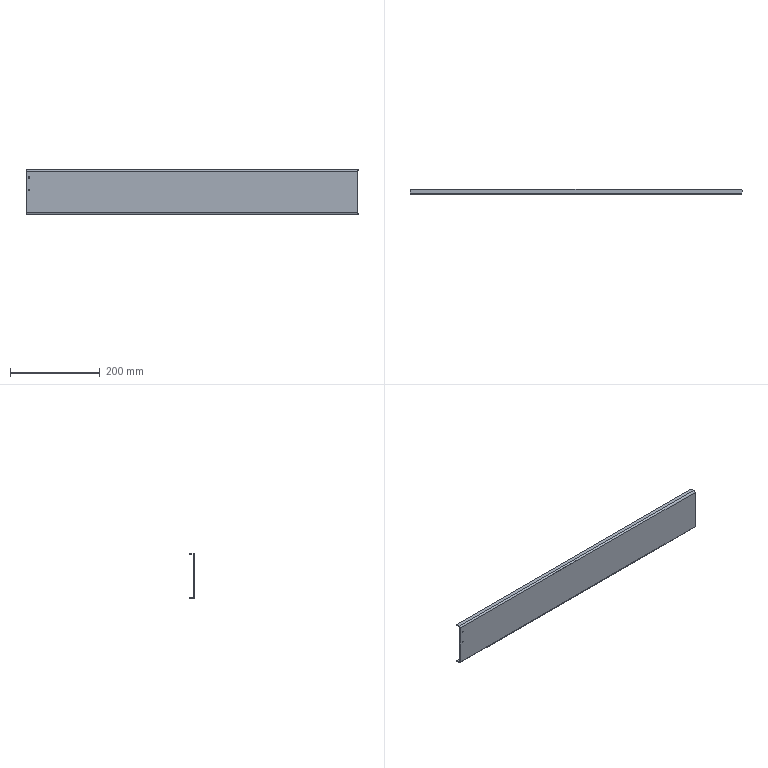Part | SolidWorks | features HoleWzd 2, EdgeFlange 1, Fillet 1, FlatPattern 1, SMBaseFlange 1, SheetMetal 1 | 1 solid | 40 faces | box 740 x 12 x 100 mm | volume 174224 mm3 | cylinder 22 | plane 18 | commonest cylinder face diameters 4.5 x10 3.3 x4 4 x4 3 x2 7 x2
STEP:
#1=CARTESIAN_POINT('',(-363.,-2.,3.35));
#2=VERTEX_POINT('',#1);
#3=CARTESIAN_POINT('',(-363.,-2.,6.65));
#4=VERTEX_POINT('',#3);
#5=CARTESIAN_POINT('',(-363.,-2.,5.));
#6=DIRECTION('',(0.,1.,0.));
#7=DIRECTION('',(0.,0.,1.));
#8=AXIS2_PLACEMENT_3D('',#5,#6,#7);
#9=CIRCLE('',#8,1.65);
#10=EDGE_CURVE('',#2,#4,#9,.T.);
#11=ORIENTED_EDGE('',*,*,#10,.F.);
#12=CARTESIAN_POINT('',(-363.,0.,3.35));
#13=VERTEX_POINT('',#12);
#14=CARTESIAN_POINT('',(-363.,0.,3.35));
#15=DIRECTION('',(0.,1.,0.));
#16=VECTOR('',#15,1000.);
#17=LINE('',#14,#16);
#18=EDGE_CURVE('',#2,#13,#17,.T.);
#19=ORIENTED_EDGE('',*,*,#18,.T.);
#20=CARTESIAN_POINT('',(-363.,0.,6.65));
#21=VERTEX_POINT('',#20);
#22=CARTESIAN_POINT('',(-363.,0.,5.));
#23=DIRECTION('',(0.,1.,0.));
#24=DIRECTION('',(0.,0.,1.));
#25=AXIS2_PLACEMENT_3D('',#22,#23,#24);
#26=CIRCLE('',#25,1.65);
#27=EDGE_CURVE('',#13,#21,#26,.T.);
#28=ORIENTED_EDGE('',*,*,#27,.T.);
#29=CARTESIAN_POINT('',(-363.,0.,6.65));
#30=DIRECTION('',(0.,1.,0.));
#31=VECTOR('',#30,1000.);
#32=LINE('',#29,#31);
#33=EDGE_CURVE('',#4,#21,#32,.T.);
#34=ORIENTED_EDGE('',*,*,#33,.F.);
#35=EDGE_LOOP('',(#11,#19,#28,#34));
#36=FACE_OUTER_BOUND('',#35,.T.);
#37=CARTESIAN_POINT('',(-363.,0.,5.));
#38=DIRECTION('',(0.,1.,0.));
#39=DIRECTION('',(0.,0.,1.));
#40=AXIS2_PLACEMENT_3D('',#37,#38,#39);
#41=CYLINDRICAL_SURFACE('',#40,1.65);
#42=ADVANCED_FACE('',(#36),#41,.F.);
#43=CARTESIAN_POINT('',(-363.,-2.,30.35));
#44=VERTEX_POINT('',#43);
#45=CARTESIAN_POINT('',(-363.,-2.,33.65));
#46=VERTEX_POINT('',#45);
#47=CARTESIAN_POINT('',(-363.,-2.,32.));
#48=DIRECTION('',(0.,1.,0.));
#49=DIRECTION('',(0.,0.,1.));
#50=AXIS2_PLACEMENT_3D('',#47,#48,#49);
#51=CIRCLE('',#50,1.65);
#52=EDGE_CURVE('',#44,#46,#51,.T.);
#53=ORIENTED_EDGE('',*,*,#52,.F.);
#54=CARTESIAN_POINT('',(-363.,0.,30.35));
#55=VERTEX_POINT('',#54);
#56=CARTESIAN_POINT('',(-363.,0.,30.35));
#57=DIRECTION('',(0.,1.,0.));
#58=VECTOR('',#57,1000.);
#59=LINE('',#56,#58);
#60=EDGE_CURVE('',#44,#55,#59,.T.);
#61=ORIENTED_EDGE('',*,*,#60,.T.);
#62=CARTESIAN_POINT('',(-363.,0.,33.65));
#63=VERTEX_POINT('',#62);
#64=CARTESIAN_POINT('',(-363.,0.,32.));
#65=DIRECTION('',(0.,1.,0.));
#66=DIRECTION('',(0.,0.,1.));
#67=AXIS2_PLACEMENT_3D('',#64,#65,#66);
#68=CIRCLE('',#67,1.65);
#69=EDGE_CURVE('',#55,#63,#68,.T.);
#70=ORIENTED_EDGE('',*,*,#69,.T.);
#71=CARTESIAN_POINT('',(-363.,0.,33.65));
#72=DIRECTION('',(0.,1.,0.));
#73=VECTOR('',#72,1000.);
#74=LINE('',#71,#73);
#75=EDGE_CURVE('',#46,#63,#74,.T.);
#76=ORIENTED_EDGE('',*,*,#75,.F.);
#77=EDGE_LOOP('',(#53,#61,#70,#76));
#78=FACE_OUTER_BOUND('',#77,.T.);
#79=CARTESIAN_POINT('',(-363.,0.,32.));
#80=DIRECTION('',(0.,1.,0.));
#81=DIRECTION('',(0.,0.,1.));
#82=AXIS2_PLACEMENT_3D('',#79,#80,#81);
#83=CYLINDRICAL_SURFACE('',#82,1.65);
#84=ADVANCED_FACE('',(#78),#83,.F.);
#85=CARTESIAN_POINT('',(-302.25,6.,-50.));
#86=VERTEX_POINT('',#85);
#87=CARTESIAN_POINT('',(-297.75,6.,-50.));
#88=VERTEX_POINT('',#87);
#89=CARTESIAN_POINT('',(-300.,6.,-50.));
#90=DIRECTION('',(0.,0.,1.));
#91=DIRECTION('',(1.,0.,0.));
#92=AXIS2_PLACEMENT_3D('',#89,#90,#91);
#93=CIRCLE('',#92,2.25);
#94=EDGE_CURVE('',#86,#88,#93,.T.);
#95=ORIENTED_EDGE('',*,*,#94,.F.);
#96=CARTESIAN_POINT('',(-302.25,6.,-48.));
#97=VERTEX_POINT('',#96);
#98=CARTESIAN_POINT('',(-302.25,6.,-48.));
#99=DIRECTION('',(0.,0.,1.));
#100=VECTOR('',#99,1000.);
#101=LINE('',#98,#100);
#102=EDGE_CURVE('',#86,#97,#101,.T.);
#103=ORIENTED_EDGE('',*,*,#102,.T.);
#104=CARTESIAN_POINT('',(-297.75,6.,-48.));
#105=VERTEX_POINT('',#104);
#106=CARTESIAN_POINT('',(-300.,6.,-48.));
#107=DIRECTION('',(0.,0.,1.));
#108=DIRECTION('',(1.,0.,0.));
#109=AXIS2_PLACEMENT_3D('',#106,#107,#108);
#110=CIRCLE('',#109,2.25);
#111=EDGE_CURVE('',#97,#105,#110,.T.);
#112=ORIENTED_EDGE('',*,*,#111,.T.);
#113=CARTESIAN_POINT('',(-297.75,6.,-48.));
#114=DIRECTION('',(0.,0.,1.));
#115=VECTOR('',#114,1000.);
#116=LINE('',#113,#115);
#117=EDGE_CURVE('',#88,#105,#116,.T.);
#118=ORIENTED_EDGE('',*,*,#117,.F.);
#119=EDGE_LOOP('',(#95,#103,#112,#118));
#120=FACE_OUTER_BOUND('',#119,.T.);
#121=CARTESIAN_POINT('',(-300.,6.,-48.));
#122=DIRECTION('',(0.,0.,1.));
#123=DIRECTION('',(1.,0.,0.));
#124=AXIS2_PLACEMENT_3D('',#121,#122,#123);
#125=CYLINDRICAL_SURFACE('',#124,2.25);
#126=ADVANCED_FACE('',(#120),#125,.F.);
#127=CARTESIAN_POINT('',(297.75,6.,-50.));
#128=VERTEX_POINT('',#127);
#129=CARTESIAN_POINT('',(302.25,6.,-50.));
#130=VERTEX_POINT('',#129);
#131=CARTESIAN_POINT('',(300.,6.,-50.));
#132=DIRECTION('',(0.,0.,1.));
#133=DIRECTION('',(1.,0.,0.));
#134=AXIS2_PLACEMENT_3D('',#131,#132,#133);
#135=CIRCLE('',#134,2.25);
#136=EDGE_CURVE('',#128,#130,#135,.T.);
#137=ORIENTED_EDGE('',*,*,#136,.F.);
#138=CARTESIAN_POINT('',(297.75,6.,-48.));
#139=VERTEX_POINT('',#138);
#140=CARTESIAN_POINT('',(297.75,6.,-48.));
#141=DIRECTION('',(0.,0.,1.));
#142=VECTOR('',#141,1000.);
#143=LINE('',#140,#142);
#144=EDGE_CURVE('',#128,#139,#143,.T.);
#145=ORIENTED_EDGE('',*,*,#144,.T.);
#146=CARTESIAN_POINT('',(302.25,6.,-48.));
#147=VERTEX_POINT('',#146);
#148=CARTESIAN_POINT('',(300.,6.,-48.));
#149=DIRECTION('',(0.,0.,1.));
#150=DIRECTION('',(1.,0.,0.));
#151=AXIS2_PLACEMENT_3D('',#148,#149,#150);
#152=CIRCLE('',#151,2.25);
#153=EDGE_CURVE('',#139,#147,#152,.T.);
#154=ORIENTED_EDGE('',*,*,#153,.T.);
#155=CARTESIAN_POINT('',(302.25,6.,-48.));
#156=DIRECTION('',(0.,0.,1.));
#157=VECTOR('',#156,1000.);
#158=LINE('',#155,#157);
#159=EDGE_CURVE('',#130,#147,#158,.T.);
#160=ORIENTED_EDGE('',*,*,#159,.F.);
#161=EDGE_LOOP('',(#137,#145,#154,#160));
#162=FACE_OUTER_BOUND('',#161,.T.);
#163=CARTESIAN_POINT('',(300.,6.,-48.));
#164=DIRECTION('',(0.,0.,1.));
#165=DIRECTION('',(1.,0.,0.));
#166=AXIS2_PLACEMENT_3D('',#163,#164,#165);
#167=CYLINDRICAL_SURFACE('',#166,2.25);
#168=ADVANCED_FACE('',(#162),#167,.F.);
#169=CARTESIAN_POINT('',(-152.25,6.,-50.));
#170=VERTEX_POINT('',#169);
#171=CARTESIAN_POINT('',(-147.75,6.,-50.));
#172=VERTEX_POINT('',#171);
#173=CARTESIAN_POINT('',(-150.,6.,-50.));
#174=DIRECTION('',(0.,0.,1.));
#175=DIRECTION('',(1.,0.,0.));
#176=AXIS2_PLACEMENT_3D('',#173,#174,#175);
#177=CIRCLE('',#176,2.25);
#178=EDGE_CURVE('',#170,#172,#177,.T.);
#179=ORIENTED_EDGE('',*,*,#178,.F.);
#180=CARTESIAN_POINT('',(-152.25,6.,-48.));
#181=VERTEX_POINT('',#180);
#182=CARTESIAN_POINT('',(-152.25,6.,-48.));
#183=DIRECTION('',(0.,0.,1.));
#184=VECTOR('',#183,1000.);
#185=LINE('',#182,#184);
#186=EDGE_CURVE('',#170,#181,#185,.T.);
#187=ORIENTED_EDGE('',*,*,#186,.T.);
#188=CARTESIAN_POINT('',(-147.75,6.,-48.));
#189=VERTEX_POINT('',#188);
#190=CARTESIAN_POINT('',(-150.,6.,-48.));
#191=DIRECTION('',(0.,0.,1.));
#192=DIRECTION('',(1.,0.,0.));
#193=AXIS2_PLACEMENT_3D('',#190,#191,#192);
#194=CIRCLE('',#193,2.25);
#195=EDGE_CURVE('',#181,#189,#194,.T.);
#196=ORIENTED_EDGE('',*,*,#195,.T.);
#197=CARTESIAN_POINT('',(-147.75,6.,-48.));
#198=DIRECTION('',(0.,0.,1.));
#199=VECTOR('',#198,1000.);
#200=LINE('',#197,#199);
#201=EDGE_CURVE('',#172,#189,#200,.T.);
#202=ORIENTED_EDGE('',*,*,#201,.F.);
#203=EDGE_LOOP('',(#179,#187,#196,#202));
#204=FACE_OUTER_BOUND('',#203,.T.);
#205=CARTESIAN_POINT('',(-150.,6.,-48.));
#206=DIRECTION('',(0.,0.,1.));
#207=DIRECTION('',(1.,0.,0.));
#208=AXIS2_PLACEMENT_3D('',#205,#206,#207);
#209=CYLINDRICAL_SURFACE('',#208,2.25);
#210=ADVANCED_FACE('',(#204),#209,.F.);
#211=CARTESIAN_POINT('',(147.75,6.,-50.));
#212=VERTEX_POINT('',#211);
#213=CARTESIAN_POINT('',(152.25,6.,-50.));
#214=VERTEX_POINT('',#213);
#215=CARTESIAN_POINT('',(150.,6.,-50.));
#216=DIRECTION('',(0.,0.,1.));
#217=DIRECTION('',(1.,0.,0.));
#218=AXIS2_PLACEMENT_3D('',#215,#216,#217);
#219=CIRCLE('',#218,2.25);
#220=EDGE_CURVE('',#212,#214,#219,.T.);
#221=ORIENTED_EDGE('',*,*,#220,.F.);
#222=CARTESIAN_POINT('',(147.75,6.,-48.));
#223=VERTEX_POINT('',#222);
#224=CARTESIAN_POINT('',(147.75,6.,-48.));
#225=DIRECTION('',(0.,0.,1.));
#226=VECTOR('',#225,1000.);
#227=LINE('',#224,#226);
#228=EDGE_CURVE('',#212,#223,#227,.T.);
#229=ORIENTED_EDGE('',*,*,#228,.T.);
#230=CARTESIAN_POINT('',(152.25,6.,-48.));
#231=VERTEX_POINT('',#230);
#232=CARTESIAN_POINT('',(150.,6.,-48.));
#233=DIRECTION('',(0.,0.,1.));
#234=DIRECTION('',(1.,0.,0.));
#235=AXIS2_PLACEMENT_3D('',#232,#233,#234);
#236=CIRCLE('',#235,2.25);
#237=EDGE_CURVE('',#223,#231,#236,.T.);
#238=ORIENTED_EDGE('',*,*,#237,.T.);
#239=CARTESIAN_POINT('',(152.25,6.,-48.));
#240=DIRECTION('',(0.,0.,1.));
#241=VECTOR('',#240,1000.);
#242=LINE('',#239,#241);
#243=EDGE_CURVE('',#214,#231,#242,.T.);
#244=ORIENTED_EDGE('',*,*,#243,.F.);
#245=EDGE_LOOP('',(#221,#229,#238,#244));
#246=FACE_OUTER_BOUND('',#245,.T.);
#247=CARTESIAN_POINT('',(150.,6.,-48.));
#248=DIRECTION('',(0.,0.,1.));
#249=DIRECTION('',(1.,0.,0.));
#250=AXIS2_PLACEMENT_3D('',#247,#248,#249);
#251=CYLINDRICAL_SURFACE('',#250,2.25);
#252=ADVANCED_FACE('',(#246),#251,.F.);
#253=CARTESIAN_POINT('',(-2.25,6.,-50.));
#254=VERTEX_POINT('',#253);
#255=CARTESIAN_POINT('',(2.25,6.,-50.));
#256=VERTEX_POINT('',#255);
#257=CARTESIAN_POINT('',(0.,6.,-50.));
#258=DIRECTION('',(0.,0.,1.));
#259=DIRECTION('',(1.,0.,0.));
#260=AXIS2_PLACEMENT_3D('',#257,#258,#259);
#261=CIRCLE('',#260,2.25);
#262=EDGE_CURVE('',#254,#256,#261,.T.);
#263=ORIENTED_EDGE('',*,*,#262,.F.);
#264=CARTESIAN_POINT('',(-2.25,6.,-48.));
#265=VERTEX_POINT('',#264);
#266=CARTESIAN_POINT('',(-2.25,6.,-48.));
#267=DIRECTION('',(0.,0.,1.));
#268=VECTOR('',#267,1000.);
#269=LINE('',#266,#268);
#270=EDGE_CURVE('',#254,#265,#269,.T.);
#271=ORIENTED_EDGE('',*,*,#270,.T.);
#272=CARTESIAN_POINT('',(2.25,6.,-48.));
#273=VERTEX_POINT('',#272);
#274=CARTESIAN_POINT('',(0.,6.,-48.));
#275=DIRECTION('',(0.,0.,1.));
#276=DIRECTION('',(1.,0.,0.));
#277=AXIS2_PLACEMENT_3D('',#274,#275,#276);
#278=CIRCLE('',#277,2.25);
#279=EDGE_CURVE('',#265,#273,#278,.T.);
#280=ORIENTED_EDGE('',*,*,#279,.T.);
#281=CARTESIAN_POINT('',(2.25,6.,-48.));
#282=DIRECTION('',(0.,0.,1.));
#283=VECTOR('',#282,1000.);
#284=LINE('',#281,#283);
#285=EDGE_CURVE('',#256,#273,#284,.T.);
#286=ORIENTED_EDGE('',*,*,#285,.F.);
#287=EDGE_LOOP('',(#263,#271,#280,#286));
#288=FACE_OUTER_BOUND('',#287,.T.);
#289=CARTESIAN_POINT('',(0.,6.,-48.));
#290=DIRECTION('',(0.,0.,1.));
#291=DIRECTION('',(1.,0.,0.));
#292=AXIS2_PLACEMENT_3D('',#289,#290,#291);
#293=CYLINDRICAL_SURFACE('',#292,2.25);
#294=ADVANCED_FACE('',(#288),#293,.F.);
#295=CARTESIAN_POINT('',(-363.,-2.,5.));
#296=DIRECTION('',(0.,1.,0.));
#297=DIRECTION('',(0.,0.,1.));
#298=AXIS2_PLACEMENT_3D('',#295,#296,#297);
#299=CIRCLE('',#298,1.65);
#300=EDGE_CURVE('',#4,#2,#299,.T.);
#301=ORIENTED_EDGE('',*,*,#300,.T.);
#302=ORIENTED_EDGE('',*,*,#10,.T.);
#303=EDGE_LOOP('',(#301,#302));
#304=FACE_BOUND('',#303,.T.);
#305=CARTESIAN_POINT('',(-363.,-2.,32.));
#306=DIRECTION('',(0.,1.,0.));
#307=DIRECTION('',(0.,0.,1.));
#308=AXIS2_PLACEMENT_3D('',#305,#306,#307);
#309=CIRCLE('',#308,1.65);
#310=EDGE_CURVE('',#46,#44,#309,.T.);
#311=ORIENTED_EDGE('',*,*,#310,.T.);
#312=ORIENTED_EDGE('',*,*,#52,.T.);
#313=EDGE_LOOP('',(#311,#312));
#314=FACE_BOUND('',#313,.T.);
#315=CARTESIAN_POINT('',(370.,-2.,46.5));
#316=VERTEX_POINT('',#315);
#317=CARTESIAN_POINT('',(-370.,-2.,46.5));
#318=VERTEX_POINT('',#317);
#319=CARTESIAN_POINT('',(370.,-2.,46.5));
#320=DIRECTION('',(-1.,0.,0.));
#321=VECTOR('',#320,1000.);
#322=LINE('',#319,#321);
#323=EDGE_CURVE('',#316,#318,#322,.T.);
#324=ORIENTED_EDGE('',*,*,#323,.T.);
#325=CARTESIAN_POINT('',(-370.,-2.,-46.5));
#326=VERTEX_POINT('',#325);
#327=CARTESIAN_POINT('',(-370.,-2.,50.));
#328=DIRECTION('',(0.,0.,1.));
#329=VECTOR('',#328,1000.);
#330=LINE('',#327,#329);
#331=EDGE_CURVE('',#326,#318,#330,.T.);
#332=ORIENTED_EDGE('',*,*,#331,.F.);
#333=CARTESIAN_POINT('',(370.,-2.,-46.5));
#334=VERTEX_POINT('',#333);
#335=CARTESIAN_POINT('',(-370.,-2.,-46.5));
#336=DIRECTION('',(1.,0.,0.));
#337=VECTOR('',#336,1000.);
#338=LINE('',#335,#337);
#339=EDGE_CURVE('',#326,#334,#338,.T.);
#340=ORIENTED_EDGE('',*,*,#339,.T.);
#341=CARTESIAN_POINT('',(370.,-2.,50.));
#342=DIRECTION('',(0.,0.,-1.));
#343=VECTOR('',#342,1000.);
#344=LINE('',#341,#343);
#345=EDGE_CURVE('',#316,#334,#344,.T.);
#346=ORIENTED_EDGE('',*,*,#345,.F.);
#347=EDGE_LOOP('',(#324,#332,#340,#346));
#348=FACE_OUTER_BOUND('',#347,.T.);
#349=CARTESIAN_POINT('',(0.,-2.,0.));
#350=DIRECTION('',(0.,1.,0.));
#351=DIRECTION('',(0.,0.,1.));
#352=AXIS2_PLACEMENT_3D('',#349,#350,#351);
#353=PLANE('',#352);
#354=ADVANCED_FACE('',(#304,#314,#348),#353,.F.);
#355=CARTESIAN_POINT('',(-363.,0.,5.));
#356=DIRECTION('',(0.,1.,0.));
#357=DIRECTION('',(0.,0.,1.));
#358=AXIS2_PLACEMENT_3D('',#355,#356,#357);
#359=CIRCLE('',#358,1.65);
#360=EDGE_CURVE('',#21,#13,#359,.T.);
#361=ORIENTED_EDGE('',*,*,#360,.F.);
#362=ORIENTED_EDGE('',*,*,#27,.F.);
#363=EDGE_LOOP('',(#361,#362));
#364=FACE_BOUND('',#363,.T.);
#365=CARTESIAN_POINT('',(-363.,0.,32.));
#366=DIRECTION('',(0.,1.,0.));
#367=DIRECTION('',(0.,0.,1.));
#368=AXIS2_PLACEMENT_3D('',#365,#366,#367);
#369=CIRCLE('',#368,1.65);
#370=EDGE_CURVE('',#63,#55,#369,.T.);
#371=ORIENTED_EDGE('',*,*,#370,.F.);
#372=ORIENTED_EDGE('',*,*,#69,.F.);
#373=EDGE_LOOP('',(#371,#372));
#374=FACE_BOUND('',#373,.T.);
#375=CARTESIAN_POINT('',(-370.,0.,-46.5));
#376=VERTEX_POINT('',#375);
#377=CARTESIAN_POINT('',(-370.,0.,46.5));
#378=VERTEX_POINT('',#377);
#379=CARTESIAN_POINT('',(-370.,0.,50.));
#380=DIRECTION('',(0.,0.,1.));
#381=VECTOR('',#380,1000.);
#382=LINE('',#379,#381);
#383=EDGE_CURVE('',#376,#378,#382,.T.);
#384=ORIENTED_EDGE('',*,*,#383,.T.);
#385=CARTESIAN_POINT('',(370.,0.,46.5));
#386=VERTEX_POINT('',#385);
#387=CARTESIAN_POINT('',(370.,0.,46.5));
#388=DIRECTION('',(-1.,0.,0.));
#389=VECTOR('',#388,1000.);
#390=LINE('',#387,#389);
#391=EDGE_CURVE('',#386,#378,#390,.T.);
#392=ORIENTED_EDGE('',*,*,#391,.F.);
#393=CARTESIAN_POINT('',(370.,0.,-46.5));
#394=VERTEX_POINT('',#393);
#395=CARTESIAN_POINT('',(370.,0.,50.));
#396=DIRECTION('',(0.,0.,-1.));
#397=VECTOR('',#396,1000.);
#398=LINE('',#395,#397);
#399=EDGE_CURVE('',#386,#394,#398,.T.);
#400=ORIENTED_EDGE('',*,*,#399,.T.);
#401=CARTESIAN_POINT('',(-370.,0.,-46.5));
#402=DIRECTION('',(1.,0.,0.));
#403=VECTOR('',#402,1000.);
#404=LINE('',#401,#403);
#405=EDGE_CURVE('',#376,#394,#404,.T.);
#406=ORIENTED_EDGE('',*,*,#405,.F.);
#407=EDGE_LOOP('',(#384,#392,#400,#406));
#408=FACE_OUTER_BOUND('',#407,.T.);
#409=CARTESIAN_POINT('',(0.,0.,0.));
#410=DIRECTION('',(0.,1.,0.));
#411=DIRECTION('',(0.,0.,1.));
#412=AXIS2_PLACEMENT_3D('',#409,#410,#411);
#413=PLANE('',#412);
#414=ADVANCED_FACE('',(#364,#374,#408),#413,.T.);
#415=ORIENTED_EDGE('',*,*,#399,.F.);
#416=CARTESIAN_POINT('',(370.,0.,46.5));
#417=DIRECTION('',(0.,-1.,0.));
#418=VECTOR('',#417,1000.);
#419=LINE('',#416,#418);
#420=EDGE_CURVE('',#386,#316,#419,.T.);
#421=ORIENTED_EDGE('',*,*,#420,.T.);
#422=ORIENTED_EDGE('',*,*,#345,.T.);
#423=CARTESIAN_POINT('',(370.,0.,-46.5));
#424=DIRECTION('',(0.,-1.,0.));
#425=VECTOR('',#424,1000.);
#426=LINE('',#423,#425);
#427=EDGE_CURVE('',#394,#334,#426,.T.);
#428=ORIENTED_EDGE('',*,*,#427,.F.);
#429=EDGE_LOOP('',(#415,#421,#422,#428));
#430=FACE_OUTER_BOUND('',#429,.T.);
#431=CARTESIAN_POINT('',(370.,-2.,50.));
#432=DIRECTION('',(1.,0.,0.));
#433=DIRECTION('',(0.,0.,-1.));
#434=AXIS2_PLACEMENT_3D('',#431,#432,#433);
#435=PLANE('',#434);
#436=ADVANCED_FACE('',(#430),#435,.T.);
#437=CARTESIAN_POINT('',(-370.,0.,46.5));
#438=DIRECTION('',(0.,-1.,0.));
#439=VECTOR('',#438,1000.);
#440=LINE('',#437,#439);
#441=EDGE_CURVE('',#378,#318,#440,.T.);
#442=ORIENTED_EDGE('',*,*,#441,.F.);
#443=ORIENTED_EDGE('',*,*,#383,.F.);
#444=CARTESIAN_POINT('',(-370.,0.,-46.5));
#445=DIRECTION('',(0.,-1.,0.));
#446=VECTOR('',#445,1000.);
#447=LINE('',#444,#446);
#448=EDGE_CURVE('',#376,#326,#447,.T.);
#449=ORIENTED_EDGE('',*,*,#448,.T.);
#450=ORIENTED_EDGE('',*,*,#331,.T.);
#451=EDGE_LOOP('',(#442,#443,#449,#450));
#452=FACE_OUTER_BOUND('',#451,.T.);
#453=CARTESIAN_POINT('',(-370.,-2.,50.));
#454=DIRECTION('',(-1.,0.,0.));
#455=DIRECTION('',(0.,0.,1.));
#456=AXIS2_PLACEMENT_3D('',#453,#454,#455);
#457=PLANE('',#456);
#458=ADVANCED_FACE('',(#452),#457,.T.);
#459=CARTESIAN_POINT('',(370.,1.5,-48.));
#460=VERTEX_POINT('',#459);
#461=CARTESIAN_POINT('',(370.,1.5,-50.));
#462=VERTEX_POINT('',#461);
#463=CARTESIAN_POINT('',(370.,1.5,-50.));
#464=DIRECTION('',(0.,0.,-1.));
#465=VECTOR('',#464,1000.);
#466=LINE('',#463,#465);
#467=EDGE_CURVE('',#460,#462,#466,.T.);
#468=ORIENTED_EDGE('',*,*,#467,.F.);
#469=CARTESIAN_POINT('',(370.,1.5,-46.5));
#470=DIRECTION('',(1.,0.,0.));
#471=DIRECTION('',(0.,-1.,0.));
#472=AXIS2_PLACEMENT_3D('',#469,#470,#471);
#473=CIRCLE('',#472,1.5);
#474=EDGE_CURVE('',#394,#460,#473,.T.);
#475=ORIENTED_EDGE('',*,*,#474,.F.);
#476=ORIENTED_EDGE('',*,*,#427,.T.);
#477=CARTESIAN_POINT('',(370.,1.5,-46.5));
#478=DIRECTION('',(1.,0.,0.));
#479=DIRECTION('',(0.,-1.,0.));
#480=AXIS2_PLACEMENT_3D('',#477,#478,#479);
#481=CIRCLE('',#480,3.5);
#482=EDGE_CURVE('',#334,#462,#481,.T.);
#483=ORIENTED_EDGE('',*,*,#482,.T.);
#484=EDGE_LOOP('',(#468,#475,#476,#483));
#485=FACE_OUTER_BOUND('',#484,.T.);
#486=CARTESIAN_POINT('',(370.,1.5,-46.5));
#487=DIRECTION('',(1.,0.,0.));
#488=DIRECTION('',(0.,1.,0.));
#489=AXIS2_PLACEMENT_3D('',#486,#487,#488);
#490=PLANE('',#489);
#491=ADVANCED_FACE('',(#485),#490,.T.);
#492=CARTESIAN_POINT('',(-370.,1.5,-48.));
#493=VERTEX_POINT('',#492);
#494=CARTESIAN_POINT('',(-370.,1.5,-46.5));
#495=DIRECTION('',(-1.,0.,0.));
#496=DIRECTION('',(0.,-1.,0.));
#497=AXIS2_PLACEMENT_3D('',#494,#495,#496);
#498=CIRCLE('',#497,1.5);
#499=EDGE_CURVE('',#493,#376,#498,.T.);
#500=ORIENTED_EDGE('',*,*,#499,.F.);
#501=CARTESIAN_POINT('',(-370.,1.5,-50.));
#502=VERTEX_POINT('',#501);
#503=CARTESIAN_POINT('',(-370.,1.5,-48.));
#504=DIRECTION('',(0.,0.,-1.));
#505=VECTOR('',#504,1000.);
#506=LINE('',#503,#505);
#507=EDGE_CURVE('',#493,#502,#506,.T.);
#508=ORIENTED_EDGE('',*,*,#507,.T.);
#509=CARTESIAN_POINT('',(-370.,1.5,-46.5));
#510=DIRECTION('',(-1.,0.,0.));
#511=DIRECTION('',(0.,-1.,0.));
#512=AXIS2_PLACEMENT_3D('',#509,#510,#511);
#513=CIRCLE('',#512,3.5);
#514=EDGE_CURVE('',#502,#326,#513,.T.);
#515=ORIENTED_EDGE('',*,*,#514,.T.);
#516=ORIENTED_EDGE('',*,*,#448,.F.);
#517=EDGE_LOOP('',(#500,#508,#515,#516));
#518=FACE_OUTER_BOUND('',#517,.T.);
#519=CARTESIAN_POINT('',(-370.,1.5,-46.5));
#520=DIRECTION('',(1.,0.,0.));
#521=DIRECTION('',(0.,1.,0.));
#522=AXIS2_PLACEMENT_3D('',#519,#520,#521);
#523=PLANE('',#522);
#524=ADVANCED_FACE('',(#518),#523,.F.);
#525=ORIENTED_EDGE('',*,*,#339,.F.);
#526=ORIENTED_EDGE('',*,*,#514,.F.);
#527=CARTESIAN_POINT('',(370.,1.5,-50.));
#528=DIRECTION('',(1.,0.,0.));
#529=VECTOR('',#528,1000.);
#530=LINE('',#527,#529);
#531=EDGE_CURVE('',#502,#462,#530,.T.);
#532=ORIENTED_EDGE('',*,*,#531,.T.);
#533=ORIENTED_EDGE('',*,*,#482,.F.);
#534=EDGE_LOOP('',(#525,#526,#532,#533));
#535=FACE_OUTER_BOUND('',#534,.T.);
#536=CARTESIAN_POINT('',(-370.,1.5,-46.5));
#537=DIRECTION('',(-1.,0.,0.));
#538=DIRECTION('',(0.,0.,-1.));
#539=AXIS2_PLACEMENT_3D('',#536,#537,#538);
#540=CYLINDRICAL_SURFACE('',#539,3.5);
#541=ADVANCED_FACE('',(#535),#540,.T.);
#542=ORIENTED_EDGE('',*,*,#405,.T.);
#543=ORIENTED_EDGE('',*,*,#474,.T.);
#544=CARTESIAN_POINT('',(370.,1.5,-48.));
#545=DIRECTION('',(-1.,0.,0.));
#546=VECTOR('',#545,1000.);
#547=LINE('',#544,#546);
#548=EDGE_CURVE('',#460,#493,#547,.T.);
#549=ORIENTED_EDGE('',*,*,#548,.T.);
#550=ORIENTED_EDGE('',*,*,#499,.T.);
#551=EDGE_LOOP('',(#542,#543,#549,#550));
#552=FACE_OUTER_BOUND('',#551,.T.);
#553=CARTESIAN_POINT('',(-370.,1.5,-46.5));
#554=DIRECTION('',(-1.,0.,0.));
#555=DIRECTION('',(0.,0.,-1.));
#556=AXIS2_PLACEMENT_3D('',#553,#554,#555);
#557=CYLINDRICAL_SURFACE('',#556,1.5);
#558=ADVANCED_FACE('',(#552),#557,.F.);
#559=CARTESIAN_POINT('',(370.,8.,-50.));
#560=VERTEX_POINT('',#559);
#561=CARTESIAN_POINT('',(370.,0.,-50.));
#562=DIRECTION('',(0.,-1.,0.));
#563=VECTOR('',#562,1000.);
#564=LINE('',#561,#563);
#565=EDGE_CURVE('',#560,#462,#564,.T.);
#566=ORIENTED_EDGE('',*,*,#565,.F.);
#567=CARTESIAN_POINT('',(370.,8.,-48.));
#568=VERTEX_POINT('',#567);
#569=CARTESIAN_POINT('',(370.,8.,-50.));
#570=DIRECTION('',(0.,0.,1.));
#571=VECTOR('',#570,1000.);
#572=LINE('',#569,#571);
#573=EDGE_CURVE('',#560,#568,#572,.T.);
#574=ORIENTED_EDGE('',*,*,#573,.T.);
#575=CARTESIAN_POINT('',(370.,0.,-48.));
#576=DIRECTION('',(0.,-1.,0.));
#577=VECTOR('',#576,1000.);
#578=LINE('',#575,#577);
#579=EDGE_CURVE('',#568,#460,#578,.T.);
#580=ORIENTED_EDGE('',*,*,#579,.T.);
#581=ORIENTED_EDGE('',*,*,#467,.T.);
#582=EDGE_LOOP('',(#566,#574,#580,#581));
#583=FACE_OUTER_BOUND('',#582,.T.);
#584=CARTESIAN_POINT('',(370.,0.,-50.));
#585=DIRECTION('',(-1.,0.,0.));
#586=DIRECTION('',(0.,-1.,0.));
#587=AXIS2_PLACEMENT_3D('',#584,#585,#586);
#588=PLANE('',#587);
#589=ADVANCED_FACE('',(#583),#588,.F.);
#590=CARTESIAN_POINT('',(-370.,8.,-48.));
#591=VERTEX_POINT('',#590);
#592=CARTESIAN_POINT('',(-370.,10.,-48.));
#593=DIRECTION('',(0.,1.,0.));
#594=VECTOR('',#593,1000.);
#595=LINE('',#592,#594);
#596=EDGE_CURVE('',#493,#591,#595,.T.);
#597=ORIENTED_EDGE('',*,*,#596,.T.);
#598=CARTESIAN_POINT('',(-370.,8.,-50.));
#599=VERTEX_POINT('',#598);
#600=CARTESIAN_POINT('',(-370.,8.,-50.));
#601=DIRECTION('',(0.,0.,-1.));
#602=VECTOR('',#601,1000.);
#603=LINE('',#600,#602);
#604=EDGE_CURVE('',#591,#599,#603,.T.);
#605=ORIENTED_EDGE('',*,*,#604,.T.);
#606=CARTESIAN_POINT('',(-370.,0.,-50.));
#607=DIRECTION('',(0.,1.,0.));
#608=VECTOR('',#607,1000.);
#609=LINE('',#606,#608);
#610=EDGE_CURVE('',#502,#599,#609,.T.);
#611=ORIENTED_EDGE('',*,*,#610,.F.);
#612=ORIENTED_EDGE('',*,*,#507,.F.);
#613=EDGE_LOOP('',(#597,#605,#611,#612));
#614=FACE_OUTER_BOUND('',#613,.T.);
#615=CARTESIAN_POINT('',(-370.,10.,-50.));
#616=DIRECTION('',(1.,0.,0.));
#617=DIRECTION('',(0.,1.,0.));
#618=AXIS2_PLACEMENT_3D('',#615,#616,#617);
#619=PLANE('',#618);
#620=ADVANCED_FACE('',(#614),#619,.F.);
#621=CARTESIAN_POINT('',(-300.,6.,-50.));
#622=DIRECTION('',(0.,0.,1.));
#623=DIRECTION('',(1.,0.,0.));
#624=AXIS2_PLACEMENT_3D('',#621,#622,#623);
#625=CIRCLE('',#624,2.25);
#626=EDGE_CURVE('',#88,#86,#625,.T.);
#627=ORIENTED_EDGE('',*,*,#626,.T.);
#628=ORIENTED_EDGE('',*,*,#94,.T.);
#629=EDGE_LOOP('',(#627,#628));
#630=FACE_BOUND('',#629,.T.);
#631=CARTESIAN_POINT('',(300.,6.,-50.));
#632=DIRECTION('',(0.,0.,1.));
#633=DIRECTION('',(1.,0.,0.));
#634=AXIS2_PLACEMENT_3D('',#631,#632,#633);
#635=CIRCLE('',#634,2.25);
#636=EDGE_CURVE('',#130,#128,#635,.T.);
#637=ORIENTED_EDGE('',*,*,#636,.T.);
#638=ORIENTED_EDGE('',*,*,#136,.T.);
#639=EDGE_LOOP('',(#637,#638));
#640=FACE_BOUND('',#639,.T.);
#641=CARTESIAN_POINT('',(-150.,6.,-50.));
#642=DIRECTION('',(0.,0.,1.));
#643=DIRECTION('',(1.,0.,0.));
#644=AXIS2_PLACEMENT_3D('',#641,#642,#643);
#645=CIRCLE('',#644,2.25);
#646=EDGE_CURVE('',#172,#170,#645,.T.);
#647=ORIENTED_EDGE('',*,*,#646,.T.);
#648=ORIENTED_EDGE('',*,*,#178,.T.);
#649=EDGE_LOOP('',(#647,#648));
#650=FACE_BOUND('',#649,.T.);
#651=CARTESIAN_POINT('',(150.,6.,-50.));
#652=DIRECTION('',(0.,0.,1.));
#653=DIRECTION('',(1.,0.,0.));
#654=AXIS2_PLACEMENT_3D('',#651,#652,#653);
#655=CIRCLE('',#654,2.25);
#656=EDGE_CURVE('',#214,#212,#655,.T.);
#657=ORIENTED_EDGE('',*,*,#656,.T.);
#658=ORIENTED_EDGE('',*,*,#220,.T.);
#659=EDGE_LOOP('',(#657,#658));
#660=FACE_BOUND('',#659,.T.);
#661=CARTESIAN_POINT('',(0.,6.,-50.));
#662=DIRECTION('',(0.,0.,1.));
#663=DIRECTION('',(1.,0.,0.));
#664=AXIS2_PLACEMENT_3D('',#661,#662,#663);
#665=CIRCLE('',#664,2.25);
#666=EDGE_CURVE('',#256,#254,#665,.T.);
#667=ORIENTED_EDGE('',*,*,#666,.T.);
#668=ORIENTED_EDGE('',*,*,#262,.T.);
#669=EDGE_LOOP('',(#667,#668));
#670=FACE_BOUND('',#669,.T.);
#671=CARTESIAN_POINT('',(-368.,10.,-50.));
#672=VERTEX_POINT('',#671);
#673=CARTESIAN_POINT('',(368.,10.,-50.));
#674=VERTEX_POINT('',#673);
#675=CARTESIAN_POINT('',(0.,10.,-50.));
#676=DIRECTION('',(1.,0.,0.));
#677=VECTOR('',#676,1000.);
#678=LINE('',#675,#677);
#679=EDGE_CURVE('',#672,#674,#678,.T.);
#680=ORIENTED_EDGE('',*,*,#679,.T.);
#681=CARTESIAN_POINT('',(368.,8.,-50.));
#682=DIRECTION('',(0.,0.,-1.));
#683=DIRECTION('',(0.,-1.,0.));
#684=AXIS2_PLACEMENT_3D('',#681,#682,#683);
#685=CIRCLE('',#684,2.);
#686=EDGE_CURVE('',#674,#560,#685,.T.);
#687=ORIENTED_EDGE('',*,*,#686,.T.);
#688=ORIENTED_EDGE('',*,*,#565,.T.);
#689=ORIENTED_EDGE('',*,*,#531,.F.);
#690=ORIENTED_EDGE('',*,*,#610,.T.);
#691=CARTESIAN_POINT('',(-368.,8.,-50.));
#692=DIRECTION('',(0.,0.,-1.));
#693=DIRECTION('',(0.,-1.,0.));
#694=AXIS2_PLACEMENT_3D('',#691,#692,#693);
#695=CIRCLE('',#694,2.);
#696=EDGE_CURVE('',#599,#672,#695,.T.);
#697=ORIENTED_EDGE('',*,*,#696,.T.);
#698=EDGE_LOOP('',(#680,#687,#688,#689,#690,#697));
#699=FACE_OUTER_BOUND('',#698,.T.);
#700=CARTESIAN_POINT('',(0.,0.,-50.));
#701=DIRECTION('',(0.,0.,1.));
#702=DIRECTION('',(0.,-1.,0.));
#703=AXIS2_PLACEMENT_3D('',#700,#701,#702);
#704=PLANE('',#703);
#705=ADVANCED_FACE('',(#630,#640,#650,#660,#670,#699),#704,.F.);
#706=CARTESIAN_POINT('',(-300.,6.,-48.));
#707=DIRECTION('',(0.,0.,1.));
#708=DIRECTION('',(1.,0.,0.));
#709=AXIS2_PLACEMENT_3D('',#706,#707,#708);
#710=CIRCLE('',#709,2.25);
#711=EDGE_CURVE('',#105,#97,#710,.T.);
#712=ORIENTED_EDGE('',*,*,#711,.F.);
#713=ORIENTED_EDGE('',*,*,#111,.F.);
#714=EDGE_LOOP('',(#712,#713));
#715=FACE_BOUND('',#714,.T.);
#716=CARTESIAN_POINT('',(300.,6.,-48.));
#717=DIRECTION('',(0.,0.,1.));
#718=DIRECTION('',(1.,0.,0.));
#719=AXIS2_PLACEMENT_3D('',#716,#717,#718);
#720=CIRCLE('',#719,2.25);
#721=EDGE_CURVE('',#147,#139,#720,.T.);
#722=ORIENTED_EDGE('',*,*,#721,.F.);
#723=ORIENTED_EDGE('',*,*,#153,.F.);
#724=EDGE_LOOP('',(#722,#723));
#725=FACE_BOUND('',#724,.T.);
#726=CARTESIAN_POINT('',(-150.,6.,-48.));
#727=DIRECTION('',(0.,0.,1.));
#728=DIRECTION('',(1.,0.,0.));
#729=AXIS2_PLACEMENT_3D('',#726,#727,#728);
#730=CIRCLE('',#729,2.25);
#731=EDGE_CURVE('',#189,#181,#730,.T.);
#732=ORIENTED_EDGE('',*,*,#731,.F.);
#733=ORIENTED_EDGE('',*,*,#195,.F.);
#734=EDGE_LOOP('',(#732,#733));
#735=FACE_BOUND('',#734,.T.);
#736=CARTESIAN_POINT('',(150.,6.,-48.));
#737=DIRECTION('',(0.,0.,1.));
#738=DIRECTION('',(1.,0.,0.));
#739=AXIS2_PLACEMENT_3D('',#736,#737,#738);
#740=CIRCLE('',#739,2.25);
#741=EDGE_CURVE('',#231,#223,#740,.T.);
#742=ORIENTED_EDGE('',*,*,#741,.F.);
#743=ORIENTED_EDGE('',*,*,#237,.F.);
#744=EDGE_LOOP('',(#742,#743));
#745=FACE_BOUND('',#744,.T.);
#746=CARTESIAN_POINT('',(0.,6.,-48.));
#747=DIRECTION('',(0.,0.,1.));
#748=DIRECTION('',(1.,0.,0.));
#749=AXIS2_PLACEMENT_3D('',#746,#747,#748);
#750=CIRCLE('',#749,2.25);
#751=EDGE_CURVE('',#273,#265,#750,.T.);
#752=ORIENTED_EDGE('',*,*,#751,.F.);
#753=ORIENTED_EDGE('',*,*,#279,.F.);
#754=EDGE_LOOP('',(#752,#753));
#755=FACE_BOUND('',#754,.T.);
#756=ORIENTED_EDGE('',*,*,#579,.F.);
#757=CARTESIAN_POINT('',(368.,10.,-48.));
#758=VERTEX_POINT('',#757);
#759=CARTESIAN_POINT('',(368.,8.,-48.));
#760=DIRECTION('',(0.,0.,1.));
#761=DIRECTION('',(0.,-1.,0.));
#762=AXIS2_PLACEMENT_3D('',#759,#760,#761);
#763=CIRCLE('',#762,2.);
#764=EDGE_CURVE('',#568,#758,#763,.T.);
#765=ORIENTED_EDGE('',*,*,#764,.T.);
#766=CARTESIAN_POINT('',(-368.,10.,-48.));
#767=VERTEX_POINT('',#766);
#768=CARTESIAN_POINT('',(370.,10.,-48.));
#769=DIRECTION('',(1.,0.,0.));
#770=VECTOR('',#769,1000.);
#771=LINE('',#768,#770);
#772=EDGE_CURVE('',#767,#758,#771,.T.);
#773=ORIENTED_EDGE('',*,*,#772,.F.);
#774=CARTESIAN_POINT('',(-368.,8.,-48.));
#775=DIRECTION('',(0.,0.,1.));
#776=DIRECTION('',(0.,-1.,0.));
#777=AXIS2_PLACEMENT_3D('',#774,#775,#776);
#778=CIRCLE('',#777,2.);
#779=EDGE_CURVE('',#767,#591,#778,.T.);
#780=ORIENTED_EDGE('',*,*,#779,.T.);
#781=ORIENTED_EDGE('',*,*,#596,.F.);
#782=ORIENTED_EDGE('',*,*,#548,.F.);
#783=EDGE_LOOP('',(#756,#765,#773,#780,#781,#782));
#784=FACE_OUTER_BOUND('',#783,.T.);
#785=CARTESIAN_POINT('',(0.,0.,-48.));
#786=DIRECTION('',(0.,0.,1.));
#787=DIRECTION('',(0.,-1.,0.));
#788=AXIS2_PLACEMENT_3D('',#785,#786,#787);
#789=PLANE('',#788);
#790=ADVANCED_FACE('',(#715,#725,#735,#745,#755,#784),#789,.T.);
#791=ORIENTED_EDGE('',*,*,#772,.T.);
#792=CARTESIAN_POINT('',(368.,10.,-50.));
#793=DIRECTION('',(0.,0.,-1.));
#794=VECTOR('',#793,1000.);
#795=LINE('',#792,#794);
#796=EDGE_CURVE('',#758,#674,#795,.T.);
#797=ORIENTED_EDGE('',*,*,#796,.T.);
#798=ORIENTED_EDGE('',*,*,#679,.F.);
#799=CARTESIAN_POINT('',(-368.,10.,-50.));
#800=DIRECTION('',(0.,0.,1.));
#801=VECTOR('',#800,1000.);
#802=LINE('',#799,#801);
#803=EDGE_CURVE('',#672,#767,#802,.T.);
#804=ORIENTED_EDGE('',*,*,#803,.T.);
#805=EDGE_LOOP('',(#791,#797,#798,#804));
#806=FACE_OUTER_BOUND('',#805,.T.);
#807=CARTESIAN_POINT('',(370.,10.,-50.));
#808=DIRECTION('',(0.,-1.,0.));
#809=DIRECTION('',(0.,0.,-1.));
#810=AXIS2_PLACEMENT_3D('',#807,#808,#809);
#811=PLANE('',#810);
#812=ADVANCED_FACE('',(#806),#811,.F.);
#813=CARTESIAN_POINT('',(-370.,1.5,48.));
#814=VERTEX_POINT('',#813);
#815=CARTESIAN_POINT('',(-370.,1.5,50.));
#816=VERTEX_POINT('',#815);
#817=CARTESIAN_POINT('',(-370.,1.5,50.));
#818=DIRECTION('',(0.,0.,1.));
#819=VECTOR('',#818,1000.);
#820=LINE('',#817,#819);
#821=EDGE_CURVE('',#814,#816,#820,.T.);
#822=ORIENTED_EDGE('',*,*,#821,.F.);
#823=CARTESIAN_POINT('',(-370.,1.5,46.5));
#824=DIRECTION('',(-1.,0.,0.));
#825=DIRECTION('',(0.,0.,-1.));
#826=AXIS2_PLACEMENT_3D('',#823,#824,#825);
#827=CIRCLE('',#826,1.5);
#828=EDGE_CURVE('',#378,#814,#827,.T.);
#829=ORIENTED_EDGE('',*,*,#828,.F.);
#830=ORIENTED_EDGE('',*,*,#441,.T.);
#831=CARTESIAN_POINT('',(-370.,1.5,46.5));
#832=DIRECTION('',(-1.,0.,0.));
#833=DIRECTION('',(0.,0.,-1.));
#834=AXIS2_PLACEMENT_3D('',#831,#832,#833);
#835=CIRCLE('',#834,3.5);
#836=EDGE_CURVE('',#318,#816,#835,.T.);
#837=ORIENTED_EDGE('',*,*,#836,.T.);
#838=EDGE_LOOP('',(#822,#829,#830,#837));
#839=FACE_OUTER_BOUND('',#838,.T.);
#840=CARTESIAN_POINT('',(-370.,1.5,46.5));
#841=DIRECTION('',(-1.,0.,0.));
#842=DIRECTION('',(0.,0.,1.));
#843=AXIS2_PLACEMENT_3D('',#840,#841,#842);
#844=PLANE('',#843);
#845=ADVANCED_FACE('',(#839),#844,.T.);
#846=CARTESIAN_POINT('',(370.,1.5,48.));
#847=VERTEX_POINT('',#846);
#848=CARTESIAN_POINT('',(370.,1.5,46.5));
#849=DIRECTION('',(1.,0.,0.));
#850=DIRECTION('',(0.,0.,-1.));
#851=AXIS2_PLACEMENT_3D('',#848,#849,#850);
#852=CIRCLE('',#851,1.5);
#853=EDGE_CURVE('',#847,#386,#852,.T.);
#854=ORIENTED_EDGE('',*,*,#853,.F.);
#855=CARTESIAN_POINT('',(370.,1.5,50.));
#856=VERTEX_POINT('',#855);
#857=CARTESIAN_POINT('',(370.,1.5,48.));
#858=DIRECTION('',(0.,0.,1.));
#859=VECTOR('',#858,1000.);
#860=LINE('',#857,#859);
#861=EDGE_CURVE('',#847,#856,#860,.T.);
#862=ORIENTED_EDGE('',*,*,#861,.T.);
#863=CARTESIAN_POINT('',(370.,1.5,46.5));
#864=DIRECTION('',(1.,0.,0.));
#865=DIRECTION('',(0.,0.,-1.));
#866=AXIS2_PLACEMENT_3D('',#863,#864,#865);
#867=CIRCLE('',#866,3.5);
#868=EDGE_CURVE('',#856,#316,#867,.T.);
#869=ORIENTED_EDGE('',*,*,#868,.T.);
#870=ORIENTED_EDGE('',*,*,#420,.F.);
#871=EDGE_LOOP('',(#854,#862,#869,#870));
#872=FACE_OUTER_BOUND('',#871,.T.);
#873=CARTESIAN_POINT('',(370.,1.5,46.5));
#874=DIRECTION('',(-1.,0.,0.));
#875=DIRECTION('',(0.,0.,1.));
#876=AXIS2_PLACEMENT_3D('',#873,#874,#875);
#877=PLANE('',#876);
#878=ADVANCED_FACE('',(#872),#877,.F.);
#879=ORIENTED_EDGE('',*,*,#323,.F.);
#880=ORIENTED_EDGE('',*,*,#868,.F.);
#881=CARTESIAN_POINT('',(-370.,1.5,50.));
#882=DIRECTION('',(-1.,0.,0.));
#883=VECTOR('',#882,1000.);
#884=LINE('',#881,#883);
#885=EDGE_CURVE('',#856,#816,#884,.T.);
#886=ORIENTED_EDGE('',*,*,#885,.T.);
#887=ORIENTED_EDGE('',*,*,#836,.F.);
#888=EDGE_LOOP('',(#879,#880,#886,#887));
#889=FACE_OUTER_BOUND('',#888,.T.);
#890=CARTESIAN_POINT('',(370.,1.5,46.5));
#891=DIRECTION('',(1.,0.,0.));
#892=DIRECTION('',(0.,0.,1.));
#893=AXIS2_PLACEMENT_3D('',#890,#891,#892);
#894=CYLINDRICAL_SURFACE('',#893,3.5);
#895=ADVANCED_FACE('',(#889),#894,.T.);
#896=ORIENTED_EDGE('',*,*,#391,.T.);
#897=ORIENTED_EDGE('',*,*,#828,.T.);
#898=CARTESIAN_POINT('',(-370.,1.5,48.));
#899=DIRECTION('',(1.,0.,0.));
#900=VECTOR('',#899,1000.);
#901=LINE('',#898,#900);
#902=EDGE_CURVE('',#814,#847,#901,.T.);
#903=ORIENTED_EDGE('',*,*,#902,.T.);
#904=ORIENTED_EDGE('',*,*,#853,.T.);
#905=EDGE_LOOP('',(#896,#897,#903,#904));
#906=FACE_OUTER_BOUND('',#905,.T.);
#907=CARTESIAN_POINT('',(370.,1.5,46.5));
#908=DIRECTION('',(1.,0.,0.));
#909=DIRECTION('',(0.,0.,1.));
#910=AXIS2_PLACEMENT_3D('',#907,#908,#909);
#911=CYLINDRICAL_SURFACE('',#910,1.5);
#912=ADVANCED_FACE('',(#906),#911,.F.);
#913=CARTESIAN_POINT('',(-370.,8.,50.));
#914=VERTEX_POINT('',#913);
#915=CARTESIAN_POINT('',(-370.,0.,50.));
#916=DIRECTION('',(0.,-1.,0.));
#917=VECTOR('',#916,1000.);
#918=LINE('',#915,#917);
#919=EDGE_CURVE('',#914,#816,#918,.T.);
#920=ORIENTED_EDGE('',*,*,#919,.F.);
#921=CARTESIAN_POINT('',(-370.,8.,48.));
#922=VERTEX_POINT('',#921);
#923=CARTESIAN_POINT('',(-370.,8.,50.));
#924=DIRECTION('',(0.,0.,-1.));
#925=VECTOR('',#924,1000.);
#926=LINE('',#923,#925);
#927=EDGE_CURVE('',#914,#922,#926,.T.);
#928=ORIENTED_EDGE('',*,*,#927,.T.);
#929=CARTESIAN_POINT('',(-370.,0.,48.));
#930=DIRECTION('',(0.,-1.,0.));
#931=VECTOR('',#930,1000.);
#932=LINE('',#929,#931);
#933=EDGE_CURVE('',#922,#814,#932,.T.);
#934=ORIENTED_EDGE('',*,*,#933,.T.);
#935=ORIENTED_EDGE('',*,*,#821,.T.);
#936=EDGE_LOOP('',(#920,#928,#934,#935));
#937=FACE_OUTER_BOUND('',#936,.T.);
#938=CARTESIAN_POINT('',(-370.,0.,50.));
#939=DIRECTION('',(1.,0.,0.));
#940=DIRECTION('',(0.,1.,0.));
#941=AXIS2_PLACEMENT_3D('',#938,#939,#940);
#942=PLANE('',#941);
#943=ADVANCED_FACE('',(#937),#942,.F.);
#944=CARTESIAN_POINT('',(370.,8.,48.));
#945=VERTEX_POINT('',#944);
#946=CARTESIAN_POINT('',(370.,10.,48.));
#947=DIRECTION('',(0.,1.,0.));
#948=VECTOR('',#947,1000.);
#949=LINE('',#946,#948);
#950=EDGE_CURVE('',#847,#945,#949,.T.);
#951=ORIENTED_EDGE('',*,*,#950,.T.);
#952=CARTESIAN_POINT('',(370.,8.,50.));
#953=VERTEX_POINT('',#952);
#954=CARTESIAN_POINT('',(370.,8.,50.));
#955=DIRECTION('',(0.,0.,1.));
#956=VECTOR('',#955,1000.);
#957=LINE('',#954,#956);
#958=EDGE_CURVE('',#945,#953,#957,.T.);
#959=ORIENTED_EDGE('',*,*,#958,.T.);
#960=CARTESIAN_POINT('',(370.,0.,50.));
#961=DIRECTION('',(0.,1.,0.));
#962=VECTOR('',#961,1000.);
#963=LINE('',#960,#962);
#964=EDGE_CURVE('',#856,#953,#963,.T.);
#965=ORIENTED_EDGE('',*,*,#964,.F.);
#966=ORIENTED_EDGE('',*,*,#861,.F.);
#967=EDGE_LOOP('',(#951,#959,#965,#966));
#968=FACE_OUTER_BOUND('',#967,.T.);
#969=CARTESIAN_POINT('',(370.,10.,50.));
#970=DIRECTION('',(-1.,0.,0.));
#971=DIRECTION('',(0.,-1.,0.));
#972=AXIS2_PLACEMENT_3D('',#969,#970,#971);
#973=PLANE('',#972);
#974=ADVANCED_FACE('',(#968),#973,.F.);
#975=CARTESIAN_POINT('',(368.,10.,50.));
#976=VERTEX_POINT('',#975);
#977=CARTESIAN_POINT('',(-368.,10.,50.));
#978=VERTEX_POINT('',#977);
#979=CARTESIAN_POINT('',(0.,10.,50.));
#980=DIRECTION('',(-1.,0.,0.));
#981=VECTOR('',#980,1000.);
#982=LINE('',#979,#981);
#983=EDGE_CURVE('',#976,#978,#982,.T.);
#984=ORIENTED_EDGE('',*,*,#983,.T.);
#985=CARTESIAN_POINT('',(-368.,8.,50.));
#986=DIRECTION('',(0.,0.,1.));
#987=DIRECTION('',(-1.,0.,0.));
#988=AXIS2_PLACEMENT_3D('',#985,#986,#987);
#989=CIRCLE('',#988,2.);
#990=EDGE_CURVE('',#978,#914,#989,.T.);
#991=ORIENTED_EDGE('',*,*,#990,.T.);
#992=ORIENTED_EDGE('',*,*,#919,.T.);
#993=ORIENTED_EDGE('',*,*,#885,.F.);
#994=ORIENTED_EDGE('',*,*,#964,.T.);
#995=CARTESIAN_POINT('',(368.,8.,50.));
#996=DIRECTION('',(0.,0.,1.));
#997=DIRECTION('',(-1.,0.,0.));
#998=AXIS2_PLACEMENT_3D('',#995,#996,#997);
#999=CIRCLE('',#998,2.);
#1000=EDGE_CURVE('',#953,#976,#999,.T.);
#1001=ORIENTED_EDGE('',*,*,#1000,.T.);
#1002=EDGE_LOOP('',(#984,#991,#992,#993,#994,#1001));
#1003=FACE_OUTER_BOUND('',#1002,.T.);
#1004=CARTESIAN_POINT('',(0.,0.,50.));
#1005=DIRECTION('',(0.,0.,-1.));
#1006=DIRECTION('',(-1.,0.,0.));
#1007=AXIS2_PLACEMENT_3D('',#1004,#1005,#1006);
#1008=PLANE('',#1007);
#1009=ADVANCED_FACE('',(#1003),#1008,.F.);
#1010=ORIENTED_EDGE('',*,*,#933,.F.);
#1011=CARTESIAN_POINT('',(-368.,10.,48.));
#1012=VERTEX_POINT('',#1011);
#1013=CARTESIAN_POINT('',(-368.,8.,48.));
#1014=DIRECTION('',(0.,0.,-1.));
#1015=DIRECTION('',(-1.,0.,0.));
#1016=AXIS2_PLACEMENT_3D('',#1013,#1014,#1015);
#1017=CIRCLE('',#1016,2.);
#1018=EDGE_CURVE('',#922,#1012,#1017,.T.);
#1019=ORIENTED_EDGE('',*,*,#1018,.T.);
#1020=CARTESIAN_POINT('',(368.,10.,48.));
#1021=VERTEX_POINT('',#1020);
#1022=CARTESIAN_POINT('',(-370.,10.,48.));
#1023=DIRECTION('',(-1.,0.,0.));
#1024=VECTOR('',#1023,1000.);
#1025=LINE('',#1022,#1024);
#1026=EDGE_CURVE('',#1021,#1012,#1025,.T.);
#1027=ORIENTED_EDGE('',*,*,#1026,.F.);
#1028=CARTESIAN_POINT('',(368.,8.,48.));
#1029=DIRECTION('',(0.,0.,-1.));
#1030=DIRECTION('',(-1.,0.,0.));
#1031=AXIS2_PLACEMENT_3D('',#1028,#1029,#1030);
#1032=CIRCLE('',#1031,2.);
#1033=EDGE_CURVE('',#1021,#945,#1032,.T.);
#1034=ORIENTED_EDGE('',*,*,#1033,.T.);
#1035=ORIENTED_EDGE('',*,*,#950,.F.);
#1036=ORIENTED_EDGE('',*,*,#902,.F.);
#1037=EDGE_LOOP('',(#1010,#1019,#1027,#1034,#1035,#1036));
#1038=FACE_OUTER_BOUND('',#1037,.T.);
#1039=CARTESIAN_POINT('',(0.,0.,48.));
#1040=DIRECTION('',(0.,0.,-1.));
#1041=DIRECTION('',(-1.,0.,0.));
#1042=AXIS2_PLACEMENT_3D('',#1039,#1040,#1041);
#1043=PLANE('',#1042);
#1044=ADVANCED_FACE('',(#1038),#1043,.T.);
#1045=ORIENTED_EDGE('',*,*,#1026,.T.);
#1046=CARTESIAN_POINT('',(-368.,10.,50.));
#1047=DIRECTION('',(0.,0.,1.));
#1048=VECTOR('',#1047,1000.);
#1049=LINE('',#1046,#1048);
#1050=EDGE_CURVE('',#1012,#978,#1049,.T.);
#1051=ORIENTED_EDGE('',*,*,#1050,.T.);
#1052=ORIENTED_EDGE('',*,*,#983,.F.);
#1053=CARTESIAN_POINT('',(368.,10.,50.));
#1054=DIRECTION('',(0.,0.,-1.));
#1055=VECTOR('',#1054,1000.);
#1056=LINE('',#1053,#1055);
#1057=EDGE_CURVE('',#976,#1021,#1056,.T.);
#1058=ORIENTED_EDGE('',*,*,#1057,.T.);
#1059=EDGE_LOOP('',(#1045,#1051,#1052,#1058));
#1060=FACE_OUTER_BOUND('',#1059,.T.);
#1061=CARTESIAN_POINT('',(-370.,10.,50.));
#1062=DIRECTION('',(0.,-1.,0.));
#1063=DIRECTION('',(0.,0.,-1.));
#1064=AXIS2_PLACEMENT_3D('',#1061,#1062,#1063);
#1065=PLANE('',#1064);
#1066=ADVANCED_FACE('',(#1060),#1065,.F.);
#1067=ORIENTED_EDGE('',*,*,#270,.F.);
#1068=ORIENTED_EDGE('',*,*,#666,.F.);
#1069=ORIENTED_EDGE('',*,*,#285,.T.);
#1070=ORIENTED_EDGE('',*,*,#751,.T.);
#1071=EDGE_LOOP('',(#1067,#1068,#1069,#1070));
#1072=FACE_OUTER_BOUND('',#1071,.T.);
#1073=CARTESIAN_POINT('',(0.,6.,-48.));
#1074=DIRECTION('',(0.,0.,1.));
#1075=DIRECTION('',(1.,0.,0.));
#1076=AXIS2_PLACEMENT_3D('',#1073,#1074,#1075);
#1077=CYLINDRICAL_SURFACE('',#1076,2.25);
#1078=ADVANCED_FACE('',(#1072),#1077,.F.);
#1079=ORIENTED_EDGE('',*,*,#228,.F.);
#1080=ORIENTED_EDGE('',*,*,#656,.F.);
#1081=ORIENTED_EDGE('',*,*,#243,.T.);
#1082=ORIENTED_EDGE('',*,*,#741,.T.);
#1083=EDGE_LOOP('',(#1079,#1080,#1081,#1082));
#1084=FACE_OUTER_BOUND('',#1083,.T.);
#1085=CARTESIAN_POINT('',(150.,6.,-48.));
#1086=DIRECTION('',(0.,0.,1.));
#1087=DIRECTION('',(1.,0.,0.));
#1088=AXIS2_PLACEMENT_3D('',#1085,#1086,#1087);
#1089=CYLINDRICAL_SURFACE('',#1088,2.25);
#1090=ADVANCED_FACE('',(#1084),#1089,.F.);
#1091=ORIENTED_EDGE('',*,*,#186,.F.);
#1092=ORIENTED_EDGE('',*,*,#646,.F.);
#1093=ORIENTED_EDGE('',*,*,#201,.T.);
#1094=ORIENTED_EDGE('',*,*,#731,.T.);
#1095=EDGE_LOOP('',(#1091,#1092,#1093,#1094));
#1096=FACE_OUTER_BOUND('',#1095,.T.);
#1097=CARTESIAN_POINT('',(-150.,6.,-48.));
#1098=DIRECTION('',(0.,0.,1.));
#1099=DIRECTION('',(1.,0.,0.));
#1100=AXIS2_PLACEMENT_3D('',#1097,#1098,#1099);
#1101=CYLINDRICAL_SURFACE('',#1100,2.25);
#1102=ADVANCED_FACE('',(#1096),#1101,.F.);
#1103=ORIENTED_EDGE('',*,*,#144,.F.);
#1104=ORIENTED_EDGE('',*,*,#636,.F.);
#1105=ORIENTED_EDGE('',*,*,#159,.T.);
#1106=ORIENTED_EDGE('',*,*,#721,.T.);
#1107=EDGE_LOOP('',(#1103,#1104,#1105,#1106));
#1108=FACE_OUTER_BOUND('',#1107,.T.);
#1109=CARTESIAN_POINT('',(300.,6.,-48.));
#1110=DIRECTION('',(0.,0.,1.));
#1111=DIRECTION('',(1.,0.,0.));
#1112=AXIS2_PLACEMENT_3D('',#1109,#1110,#1111);
#1113=CYLINDRICAL_SURFACE('',#1112,2.25);
#1114=ADVANCED_FACE('',(#1108),#1113,.F.);
#1115=ORIENTED_EDGE('',*,*,#102,.F.);
#1116=ORIENTED_EDGE('',*,*,#626,.F.);
#1117=ORIENTED_EDGE('',*,*,#117,.T.);
#1118=ORIENTED_EDGE('',*,*,#711,.T.);
#1119=EDGE_LOOP('',(#1115,#1116,#1117,#1118));
#1120=FACE_OUTER_BOUND('',#1119,.T.);
#1121=CARTESIAN_POINT('',(-300.,6.,-48.));
#1122=DIRECTION('',(0.,0.,1.));
#1123=DIRECTION('',(1.,0.,0.));
#1124=AXIS2_PLACEMENT_3D('',#1121,#1122,#1123);
#1125=CYLINDRICAL_SURFACE('',#1124,2.25);
#1126=ADVANCED_FACE('',(#1120),#1125,.F.);
#1127=ORIENTED_EDGE('',*,*,#60,.F.);
#1128=ORIENTED_EDGE('',*,*,#310,.F.);
#1129=ORIENTED_EDGE('',*,*,#75,.T.);
#1130=ORIENTED_EDGE('',*,*,#370,.T.);
#1131=EDGE_LOOP('',(#1127,#1128,#1129,#1130));
#1132=FACE_OUTER_BOUND('',#1131,.T.);
#1133=CARTESIAN_POINT('',(-363.,0.,32.));
#1134=DIRECTION('',(0.,1.,0.));
#1135=DIRECTION('',(0.,0.,1.));
#1136=AXIS2_PLACEMENT_3D('',#1133,#1134,#1135);
#1137=CYLINDRICAL_SURFACE('',#1136,1.65);
#1138=ADVANCED_FACE('',(#1132),#1137,.F.);
#1139=ORIENTED_EDGE('',*,*,#18,.F.);
#1140=ORIENTED_EDGE('',*,*,#300,.F.);
#1141=ORIENTED_EDGE('',*,*,#33,.T.);
#1142=ORIENTED_EDGE('',*,*,#360,.T.);
#1143=EDGE_LOOP('',(#1139,#1140,#1141,#1142));
#1144=FACE_OUTER_BOUND('',#1143,.T.);
#1145=CARTESIAN_POINT('',(-363.,0.,5.));
#1146=DIRECTION('',(0.,1.,0.));
#1147=DIRECTION('',(0.,0.,1.));
#1148=AXIS2_PLACEMENT_3D('',#1145,#1146,#1147);
#1149=CYLINDRICAL_SURFACE('',#1148,1.65);
#1150=ADVANCED_FACE('',(#1144),#1149,.F.);
#1151=ORIENTED_EDGE('',*,*,#990,.F.);
#1152=ORIENTED_EDGE('',*,*,#1050,.F.);
#1153=ORIENTED_EDGE('',*,*,#1018,.F.);
#1154=ORIENTED_EDGE('',*,*,#927,.F.);
#1155=EDGE_LOOP('',(#1151,#1152,#1153,#1154));
#1156=FACE_OUTER_BOUND('',#1155,.T.);
#1157=CARTESIAN_POINT('',(-368.,8.,50.));
#1158=DIRECTION('',(0.,0.,-1.));
#1159=DIRECTION('',(-1.,0.,0.));
#1160=AXIS2_PLACEMENT_3D('',#1157,#1158,#1159);
#1161=CYLINDRICAL_SURFACE('',#1160,2.);
#1162=ADVANCED_FACE('',(#1156),#1161,.T.);
#1163=ORIENTED_EDGE('',*,*,#1000,.F.);
#1164=ORIENTED_EDGE('',*,*,#958,.F.);
#1165=ORIENTED_EDGE('',*,*,#1033,.F.);
#1166=ORIENTED_EDGE('',*,*,#1057,.F.);
#1167=EDGE_LOOP('',(#1163,#1164,#1165,#1166));
#1168=FACE_OUTER_BOUND('',#1167,.T.);
#1169=CARTESIAN_POINT('',(368.,8.,50.));
#1170=DIRECTION('',(0.,0.,-1.));
#1171=DIRECTION('',(-1.,0.,0.));
#1172=AXIS2_PLACEMENT_3D('',#1169,#1170,#1171);
#1173=CYLINDRICAL_SURFACE('',#1172,2.);
#1174=ADVANCED_FACE('',(#1168),#1173,.T.);
#1175=ORIENTED_EDGE('',*,*,#686,.F.);
#1176=ORIENTED_EDGE('',*,*,#796,.F.);
#1177=ORIENTED_EDGE('',*,*,#764,.F.);
#1178=ORIENTED_EDGE('',*,*,#573,.F.);
#1179=EDGE_LOOP('',(#1175,#1176,#1177,#1178));
#1180=FACE_OUTER_BOUND('',#1179,.T.);
#1181=CARTESIAN_POINT('',(368.,8.,-50.));
#1182=DIRECTION('',(0.,0.,1.));
#1183=DIRECTION('',(0.,-1.,0.));
#1184=AXIS2_PLACEMENT_3D('',#1181,#1182,#1183);
#1185=CYLINDRICAL_SURFACE('',#1184,2.);
#1186=ADVANCED_FACE('',(#1180),#1185,.T.);
#1187=ORIENTED_EDGE('',*,*,#696,.F.);
#1188=ORIENTED_EDGE('',*,*,#604,.F.);
#1189=ORIENTED_EDGE('',*,*,#779,.F.);
#1190=ORIENTED_EDGE('',*,*,#803,.F.);
#1191=EDGE_LOOP('',(#1187,#1188,#1189,#1190));
#1192=FACE_OUTER_BOUND('',#1191,.T.);
#1193=CARTESIAN_POINT('',(-368.,8.,-50.));
#1194=DIRECTION('',(0.,0.,1.));
#1195=DIRECTION('',(0.,-1.,0.));
#1196=AXIS2_PLACEMENT_3D('',#1193,#1194,#1195);
#1197=CYLINDRICAL_SURFACE('',#1196,2.);
#1198=ADVANCED_FACE('',(#1192),#1197,.T.);
#1199=CLOSED_SHELL('',(#42,#84,#126,#168,#210,#252,#294,#354,#414,#436,#458,#491,#524,#541,#558,#589,#620,#705,#790,#812,#845,#878,#895,#912,#943,#974,#1009,#1044,#1066,#1078,#1090,#1102,#1114,#1126,#1138,#1150,#1162,#1174,#1186,#1198));
#1200=MANIFOLD_SOLID_BREP('',#1199);
#1201=CARTESIAN_POINT('',(0.,0.,0.));
#1202=DIRECTION('',(0.,0.,1.));
#1203=DIRECTION('',(1.,0.,0.));
#1204=AXIS2_PLACEMENT_3D('',#1201,#1202,#1203);
#1205=(LENGTH_UNIT()NAMED_UNIT(*)SI_UNIT(.MILLI.,.METRE.));
#1206=UNCERTAINTY_MEASURE_WITH_UNIT(LENGTH_MEASURE(0.00001),#1205,'','');
#1207=(NAMED_UNIT(*)PLANE_ANGLE_UNIT()SI_UNIT($,.RADIAN.));
#1208=(NAMED_UNIT(*)SI_UNIT($,.STERADIAN.)SOLID_ANGLE_UNIT());
#1209=(GEOMETRIC_REPRESENTATION_CONTEXT(3)GLOBAL_UNCERTAINTY_ASSIGNED_CONTEXT((#1206))GLOBAL_UNIT_ASSIGNED_CONTEXT((#1205,#1207,#1208))REPRESENTATION_CONTEXT('',''));
#1210=ADVANCED_BREP_SHAPE_REPRESENTATION('',(#1200,#1204),#1209);